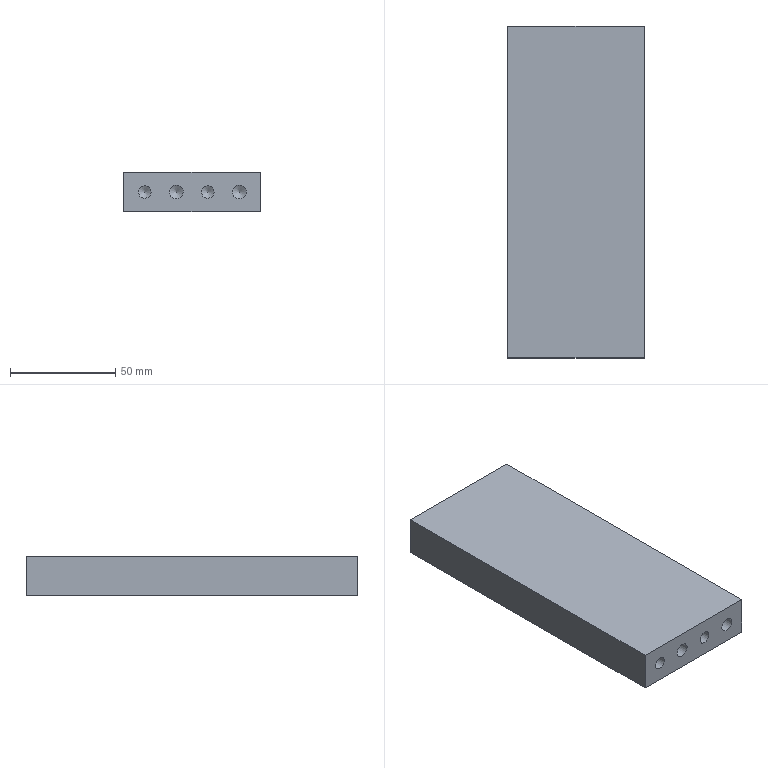Part | STEP file | SN10_006_006_SUPORTE | 1 solid | 18 faces | box 65 x 158 x 19 mm | volume 192576 mm3 | cone 6 | plane 6 | cylinder 6 | commonest cylinder face diameters 4.917 x2 6 x2 6.647 x2
STEP:
#1=CARTESIAN_POINT('',(0.,0.,0.));
#2=DIRECTION('',(0.,0.,1.));
#3=DIRECTION('',(1.,0.,0.));
#4=AXIS2_PLACEMENT_3D('',#1,#2,#3);
#5=CARTESIAN_POINT('',(286.546,-168.,375.407));
#6=VERTEX_POINT('',#5);
#7=CARTESIAN_POINT('',(283.629,-168.,377.));
#8=DIRECTION('',(0.,-1.,0.));
#9=DIRECTION('',(1.,0.,0.));
#10=AXIS2_PLACEMENT_3D('',#7,#8,#9);
#11=CIRCLE('',#10,3.324);
#12=CARTESIAN_POINT('',(283.629,-166.659,377.));
#13=DIRECTION('',(0.,-1.,0.));
#14=DIRECTION('',(0.8776,0.,-0.4794));
#15=AXIS2_PLACEMENT_3D('',#12,#13,#14);
#16=CONICAL_SURFACE('',#15,1.,1.047);
#17=CARTESIAN_POINT('',(-5.783,1.341));
#18=DIRECTION('',(1.,0.));
#19=VECTOR('',#18,1.);
#20=LINE('',#17,#19);
#21=(GEOMETRIC_REPRESENTATION_CONTEXT(2)PARAMETRIC_REPRESENTATION_CONTEXT()REPRESENTATION_CONTEXT('',''));
#22=DEFINITIONAL_REPRESENTATION('',(#20),#21);
#23=PCURVE('',#16,#22);
#24=CARTESIAN_POINT('',(283.629,-182.9,377.));
#25=DIRECTION('',(0.,1.,0.));
#26=DIRECTION('',(0.8776,0.,-0.4794));
#27=AXIS2_PLACEMENT_3D('',#24,#25,#26);
#28=CYLINDRICAL_SURFACE('',#27,3.324);
#29=CARTESIAN_POINT('',(12.066,14.9));
#30=DIRECTION('',(-1.,0.));
#31=VECTOR('',#30,1.);
#32=LINE('',#29,#31);
#33=(GEOMETRIC_REPRESENTATION_CONTEXT(2)PARAMETRIC_REPRESENTATION_CONTEXT()REPRESENTATION_CONTEXT('',''));
#34=DEFINITIONAL_REPRESENTATION('',(#32),#33);
#35=PCURVE('',#28,#34);
#36=SURFACE_CURVE('',#11,(#23,#35),.PCURVE_S1.);
#37=EDGE_CURVE('',#6,#6,#36,.T.);
#38=ORIENTED_EDGE('',*,*,#37,.F.);
#39=CARTESIAN_POINT('',(283.629,-166.081,377.));
#40=VERTEX_POINT('',#39);
#41=CARTESIAN_POINT('',(283.629,-166.081,377.));
#42=CARTESIAN_POINT('',(286.546,-168.,375.407));
#43=B_SPLINE_CURVE_WITH_KNOTS('',1,(#41,#42),.UNSPECIFIED.,.F.,.F.,(2,2),(-1.155,2.683),.PIECEWISE_BEZIER_KNOTS.);
#44=CARTESIAN_POINT('',(0.,0.));
#45=DIRECTION('',(0.,1.));
#46=VECTOR('',#45,1.);
#47=LINE('',#44,#46);
#48=(GEOMETRIC_REPRESENTATION_CONTEXT(2)PARAMETRIC_REPRESENTATION_CONTEXT()REPRESENTATION_CONTEXT('',''));
#49=DEFINITIONAL_REPRESENTATION('',(#47),#48);
#50=PCURVE('',#16,#49);
#51=CARTESIAN_POINT('',(6.283,0.));
#52=DIRECTION('',(0.,1.));
#53=VECTOR('',#52,1.);
#54=LINE('',#51,#53);
#55=(GEOMETRIC_REPRESENTATION_CONTEXT(2)PARAMETRIC_REPRESENTATION_CONTEXT()REPRESENTATION_CONTEXT('',''));
#56=DEFINITIONAL_REPRESENTATION('',(#54),#55);
#57=PCURVE('',#16,#56);
#58=SEAM_CURVE('',#43,(#50,#57),.PCURVE_S1.);
#59=EDGE_CURVE('',#40,#6,#58,.T.);
#60=ORIENTED_EDGE('',*,*,#59,.F.);
#61=ORIENTED_EDGE('',*,*,#59,.T.);
#62=EDGE_LOOP('',(#38,#60,#61));
#63=FACE_BOUND('',#62,.F.);
#64=ADVANCED_FACE('',(#63),#16,.F.);
#65=CARTESIAN_POINT('',(258.629,-183.,367.5));
#66=VERTEX_POINT('',#65);
#67=CARTESIAN_POINT('',(258.629,-25.,367.5));
#68=VERTEX_POINT('',#67);
#69=CARTESIAN_POINT('',(258.629,-183.,367.5));
#70=DIRECTION('',(0.,1.,0.));
#71=VECTOR('',#70,1.);
#72=LINE('',#69,#71);
#73=CARTESIAN_POINT('',(258.629,-183.,386.5));
#74=DIRECTION('',(-1.,0.,0.));
#75=DIRECTION('',(0.,0.,1.));
#76=AXIS2_PLACEMENT_3D('',#73,#74,#75);
#77=PLANE('',#76);
#78=CARTESIAN_POINT('',(-19.,0.));
#79=DIRECTION('',(0.,1.));
#80=VECTOR('',#79,1.);
#81=LINE('',#78,#80);
#82=(GEOMETRIC_REPRESENTATION_CONTEXT(2)PARAMETRIC_REPRESENTATION_CONTEXT()REPRESENTATION_CONTEXT('',''));
#83=DEFINITIONAL_REPRESENTATION('',(#81),#82);
#84=PCURVE('',#77,#83);
#85=CARTESIAN_POINT('',(0.,0.,367.5));
#86=DIRECTION('',(0.,0.,1.));
#87=DIRECTION('',(1.,0.,0.));
#88=AXIS2_PLACEMENT_3D('',#85,#86,#87);
#89=PLANE('',#88);
#90=CARTESIAN_POINT('',(258.629,-183.));
#91=DIRECTION('',(0.,1.));
#92=VECTOR('',#91,1.);
#93=LINE('',#90,#92);
#94=(GEOMETRIC_REPRESENTATION_CONTEXT(2)PARAMETRIC_REPRESENTATION_CONTEXT()REPRESENTATION_CONTEXT('',''));
#95=DEFINITIONAL_REPRESENTATION('',(#93),#94);
#96=PCURVE('',#89,#95);
#97=SURFACE_CURVE('',#72,(#84,#96),.PCURVE_S1.);
#98=EDGE_CURVE('',#66,#68,#97,.T.);
#99=ORIENTED_EDGE('',*,*,#98,.F.);
#100=CARTESIAN_POINT('',(258.629,-183.,386.5));
#101=VERTEX_POINT('',#100);
#102=CARTESIAN_POINT('',(258.629,-183.,386.5));
#103=DIRECTION('',(0.,0.,-1.));
#104=VECTOR('',#103,1.);
#105=LINE('',#102,#104);
#106=CARTESIAN_POINT('',(0.,0.));
#107=DIRECTION('',(-1.,0.));
#108=VECTOR('',#107,1.);
#109=LINE('',#106,#108);
#110=(GEOMETRIC_REPRESENTATION_CONTEXT(2)PARAMETRIC_REPRESENTATION_CONTEXT()REPRESENTATION_CONTEXT('',''));
#111=DEFINITIONAL_REPRESENTATION('',(#109),#110);
#112=PCURVE('',#77,#111);
#113=CARTESIAN_POINT('',(258.629,-183.,386.5));
#114=DIRECTION('',(0.,1.,0.));
#115=DIRECTION('',(0.,0.,1.));
#116=AXIS2_PLACEMENT_3D('',#113,#114,#115);
#117=PLANE('',#116);
#118=CARTESIAN_POINT('',(0.,0.));
#119=DIRECTION('',(-1.,0.));
#120=VECTOR('',#119,1.);
#121=LINE('',#118,#120);
#122=(GEOMETRIC_REPRESENTATION_CONTEXT(2)PARAMETRIC_REPRESENTATION_CONTEXT()REPRESENTATION_CONTEXT('',''));
#123=DEFINITIONAL_REPRESENTATION('',(#121),#122);
#124=PCURVE('',#117,#123);
#125=SURFACE_CURVE('',#105,(#112,#124),.PCURVE_S1.);
#126=EDGE_CURVE('',#101,#66,#125,.T.);
#127=ORIENTED_EDGE('',*,*,#126,.F.);
#128=CARTESIAN_POINT('',(258.629,-25.,386.5));
#129=VERTEX_POINT('',#128);
#130=CARTESIAN_POINT('',(258.629,-183.,386.5));
#131=DIRECTION('',(0.,1.,0.));
#132=VECTOR('',#131,1.);
#133=LINE('',#130,#132);
#134=CARTESIAN_POINT('',(0.,0.));
#135=DIRECTION('',(0.,1.));
#136=VECTOR('',#135,1.);
#137=LINE('',#134,#136);
#138=(GEOMETRIC_REPRESENTATION_CONTEXT(2)PARAMETRIC_REPRESENTATION_CONTEXT()REPRESENTATION_CONTEXT('',''));
#139=DEFINITIONAL_REPRESENTATION('',(#137),#138);
#140=PCURVE('',#77,#139);
#141=CARTESIAN_POINT('',(0.,0.,386.5));
#142=DIRECTION('',(0.,0.,1.));
#143=DIRECTION('',(1.,0.,0.));
#144=AXIS2_PLACEMENT_3D('',#141,#142,#143);
#145=PLANE('',#144);
#146=CARTESIAN_POINT('',(258.629,-183.));
#147=DIRECTION('',(0.,1.));
#148=VECTOR('',#147,1.);
#149=LINE('',#146,#148);
#150=(GEOMETRIC_REPRESENTATION_CONTEXT(2)PARAMETRIC_REPRESENTATION_CONTEXT()REPRESENTATION_CONTEXT('',''));
#151=DEFINITIONAL_REPRESENTATION('',(#149),#150);
#152=PCURVE('',#145,#151);
#153=SURFACE_CURVE('',#133,(#140,#152),.PCURVE_S1.);
#154=EDGE_CURVE('',#101,#129,#153,.T.);
#155=ORIENTED_EDGE('',*,*,#154,.T.);
#156=CARTESIAN_POINT('',(258.629,-25.,386.5));
#157=DIRECTION('',(0.,0.,-1.));
#158=VECTOR('',#157,1.);
#159=LINE('',#156,#158);
#160=CARTESIAN_POINT('',(0.,158.));
#161=DIRECTION('',(-1.,0.));
#162=VECTOR('',#161,1.);
#163=LINE('',#160,#162);
#164=(GEOMETRIC_REPRESENTATION_CONTEXT(2)PARAMETRIC_REPRESENTATION_CONTEXT()REPRESENTATION_CONTEXT('',''));
#165=DEFINITIONAL_REPRESENTATION('',(#163),#164);
#166=PCURVE('',#77,#165);
#167=CARTESIAN_POINT('',(258.629,-25.,386.5));
#168=DIRECTION('',(0.,1.,0.));
#169=DIRECTION('',(0.,0.,1.));
#170=AXIS2_PLACEMENT_3D('',#167,#168,#169);
#171=PLANE('',#170);
#172=CARTESIAN_POINT('',(0.,0.));
#173=DIRECTION('',(-1.,0.));
#174=VECTOR('',#173,1.);
#175=LINE('',#172,#174);
#176=(GEOMETRIC_REPRESENTATION_CONTEXT(2)PARAMETRIC_REPRESENTATION_CONTEXT()REPRESENTATION_CONTEXT('',''));
#177=DEFINITIONAL_REPRESENTATION('',(#175),#176);
#178=PCURVE('',#171,#177);
#179=SURFACE_CURVE('',#159,(#166,#178),.PCURVE_S1.);
#180=EDGE_CURVE('',#129,#68,#179,.T.);
#181=ORIENTED_EDGE('',*,*,#180,.T.);
#182=EDGE_LOOP('',(#99,#127,#155,#181));
#183=FACE_BOUND('',#182,.T.);
#184=ADVANCED_FACE('',(#183),#77,.T.);
#185=CARTESIAN_POINT('',(323.629,-25.,367.5));
#186=VERTEX_POINT('',#185);
#187=CARTESIAN_POINT('',(258.629,-25.,367.5));
#188=DIRECTION('',(1.,0.,0.));
#189=VECTOR('',#188,1.);
#190=LINE('',#187,#189);
#191=CARTESIAN_POINT('',(258.629,-25.));
#192=DIRECTION('',(1.,0.));
#193=VECTOR('',#192,1.);
#194=LINE('',#191,#193);
#195=(GEOMETRIC_REPRESENTATION_CONTEXT(2)PARAMETRIC_REPRESENTATION_CONTEXT()REPRESENTATION_CONTEXT('',''));
#196=DEFINITIONAL_REPRESENTATION('',(#194),#195);
#197=PCURVE('',#89,#196);
#198=CARTESIAN_POINT('',(-19.,0.));
#199=DIRECTION('',(0.,1.));
#200=VECTOR('',#199,1.);
#201=LINE('',#198,#200);
#202=(GEOMETRIC_REPRESENTATION_CONTEXT(2)PARAMETRIC_REPRESENTATION_CONTEXT()REPRESENTATION_CONTEXT('',''));
#203=DEFINITIONAL_REPRESENTATION('',(#201),#202);
#204=PCURVE('',#171,#203);
#205=SURFACE_CURVE('',#190,(#197,#204),.PCURVE_S1.);
#206=EDGE_CURVE('',#68,#186,#205,.T.);
#207=ORIENTED_EDGE('',*,*,#206,.T.);
#208=CARTESIAN_POINT('',(323.629,-183.,367.5));
#209=VERTEX_POINT('',#208);
#210=CARTESIAN_POINT('',(323.629,-25.,367.5));
#211=DIRECTION('',(0.,-1.,0.));
#212=VECTOR('',#211,1.);
#213=LINE('',#210,#212);
#214=CARTESIAN_POINT('',(323.629,-25.));
#215=DIRECTION('',(0.,-1.));
#216=VECTOR('',#215,1.);
#217=LINE('',#214,#216);
#218=(GEOMETRIC_REPRESENTATION_CONTEXT(2)PARAMETRIC_REPRESENTATION_CONTEXT()REPRESENTATION_CONTEXT('',''));
#219=DEFINITIONAL_REPRESENTATION('',(#217),#218);
#220=PCURVE('',#89,#219);
#221=CARTESIAN_POINT('',(323.629,-25.,386.5));
#222=DIRECTION('',(1.,0.,0.));
#223=DIRECTION('',(0.,0.,-1.));
#224=AXIS2_PLACEMENT_3D('',#221,#222,#223);
#225=PLANE('',#224);
#226=CARTESIAN_POINT('',(19.,0.));
#227=DIRECTION('',(0.,-1.));
#228=VECTOR('',#227,1.);
#229=LINE('',#226,#228);
#230=(GEOMETRIC_REPRESENTATION_CONTEXT(2)PARAMETRIC_REPRESENTATION_CONTEXT()REPRESENTATION_CONTEXT('',''));
#231=DEFINITIONAL_REPRESENTATION('',(#229),#230);
#232=PCURVE('',#225,#231);
#233=SURFACE_CURVE('',#213,(#220,#232),.PCURVE_S1.);
#234=EDGE_CURVE('',#186,#209,#233,.T.);
#235=ORIENTED_EDGE('',*,*,#234,.T.);
#236=CARTESIAN_POINT('',(258.629,-183.,367.5));
#237=DIRECTION('',(1.,0.,0.));
#238=VECTOR('',#237,1.);
#239=LINE('',#236,#238);
#240=CARTESIAN_POINT('',(258.629,-183.));
#241=DIRECTION('',(1.,0.));
#242=VECTOR('',#241,1.);
#243=LINE('',#240,#242);
#244=(GEOMETRIC_REPRESENTATION_CONTEXT(2)PARAMETRIC_REPRESENTATION_CONTEXT()REPRESENTATION_CONTEXT('',''));
#245=DEFINITIONAL_REPRESENTATION('',(#243),#244);
#246=PCURVE('',#89,#245);
#247=CARTESIAN_POINT('',(-19.,0.));
#248=DIRECTION('',(0.,1.));
#249=VECTOR('',#248,1.);
#250=LINE('',#247,#249);
#251=(GEOMETRIC_REPRESENTATION_CONTEXT(2)PARAMETRIC_REPRESENTATION_CONTEXT()REPRESENTATION_CONTEXT('',''));
#252=DEFINITIONAL_REPRESENTATION('',(#250),#251);
#253=PCURVE('',#117,#252);
#254=SURFACE_CURVE('',#239,(#246,#253),.PCURVE_S1.);
#255=EDGE_CURVE('',#66,#209,#254,.T.);
#256=ORIENTED_EDGE('',*,*,#255,.F.);
#257=ORIENTED_EDGE('',*,*,#98,.T.);
#258=EDGE_LOOP('',(#207,#235,#256,#257));
#259=FACE_BOUND('',#258,.T.);
#260=ADVANCED_FACE('',(#259),#89,.F.);
#261=CARTESIAN_POINT('',(301.262,-183.,375.562));
#262=VERTEX_POINT('',#261);
#263=CARTESIAN_POINT('',(298.629,-183.,377.));
#264=DIRECTION('',(0.,1.,0.));
#265=DIRECTION('',(1.,0.,0.));
#266=AXIS2_PLACEMENT_3D('',#263,#264,#265);
#267=CIRCLE('',#266,3.);
#268=CARTESIAN_POINT('',(298.629,-182.9,377.));
#269=DIRECTION('',(0.,1.,0.));
#270=DIRECTION('',(0.8776,0.,-0.4794));
#271=AXIS2_PLACEMENT_3D('',#268,#269,#270);
#272=CYLINDRICAL_SURFACE('',#271,3.);
#273=CARTESIAN_POINT('',(-0.5,-0.1));
#274=DIRECTION('',(1.,0.));
#275=VECTOR('',#274,1.);
#276=LINE('',#273,#275);
#277=(GEOMETRIC_REPRESENTATION_CONTEXT(2)PARAMETRIC_REPRESENTATION_CONTEXT()REPRESENTATION_CONTEXT('',''));
#278=DEFINITIONAL_REPRESENTATION('',(#276),#277);
#279=PCURVE('',#272,#278);
#280=CARTESIAN_POINT('',(-9.5,40.));
#281=DIRECTION('',(0.,1.));
#282=AXIS2_PLACEMENT_2D('',#280,#281);
#283=CIRCLE('',#282,3.);
#284=(GEOMETRIC_REPRESENTATION_CONTEXT(2)PARAMETRIC_REPRESENTATION_CONTEXT()REPRESENTATION_CONTEXT('',''));
#285=DEFINITIONAL_REPRESENTATION('',(#283),#284);
#286=PCURVE('',#117,#285);
#287=SURFACE_CURVE('',#267,(#279,#286),.PCURVE_S1.);
#288=EDGE_CURVE('',#262,#262,#287,.T.);
#289=ORIENTED_EDGE('',*,*,#288,.T.);
#290=CARTESIAN_POINT('',(301.262,-168.,375.562));
#291=VERTEX_POINT('',#290);
#292=CARTESIAN_POINT('',(301.262,-183.,375.562));
#293=CARTESIAN_POINT('',(301.262,-168.,375.562));
#294=B_SPLINE_CURVE_WITH_KNOTS('',1,(#292,#293),.UNSPECIFIED.,.F.,.F.,(2,2),(-0.1,14.9),.PIECEWISE_BEZIER_KNOTS.);
#295=CARTESIAN_POINT('',(6.283,0.));
#296=DIRECTION('',(0.,1.));
#297=VECTOR('',#296,1.);
#298=LINE('',#295,#297);
#299=(GEOMETRIC_REPRESENTATION_CONTEXT(2)PARAMETRIC_REPRESENTATION_CONTEXT()REPRESENTATION_CONTEXT('',''));
#300=DEFINITIONAL_REPRESENTATION('',(#298),#299);
#301=PCURVE('',#272,#300);
#302=CARTESIAN_POINT('',(0.,0.));
#303=DIRECTION('',(0.,1.));
#304=VECTOR('',#303,1.);
#305=LINE('',#302,#304);
#306=(GEOMETRIC_REPRESENTATION_CONTEXT(2)PARAMETRIC_REPRESENTATION_CONTEXT()REPRESENTATION_CONTEXT('',''));
#307=DEFINITIONAL_REPRESENTATION('',(#305),#306);
#308=PCURVE('',#272,#307);
#309=SEAM_CURVE('',#294,(#301,#308),.PCURVE_S1.);
#310=EDGE_CURVE('',#262,#291,#309,.T.);
#311=ORIENTED_EDGE('',*,*,#310,.T.);
#312=CARTESIAN_POINT('',(298.629,-168.,377.));
#313=DIRECTION('',(0.,1.,0.));
#314=DIRECTION('',(1.,0.,0.));
#315=AXIS2_PLACEMENT_3D('',#312,#313,#314);
#316=CIRCLE('',#315,3.);
#317=CARTESIAN_POINT('',(-0.5,14.9));
#318=DIRECTION('',(1.,0.));
#319=VECTOR('',#318,1.);
#320=LINE('',#317,#319);
#321=(GEOMETRIC_REPRESENTATION_CONTEXT(2)PARAMETRIC_REPRESENTATION_CONTEXT()REPRESENTATION_CONTEXT('',''));
#322=DEFINITIONAL_REPRESENTATION('',(#320),#321);
#323=PCURVE('',#272,#322);
#324=CARTESIAN_POINT('',(298.629,-166.845,377.));
#325=DIRECTION('',(0.,-1.,0.));
#326=DIRECTION('',(0.8776,0.,-0.4794));
#327=AXIS2_PLACEMENT_3D('',#324,#325,#326);
#328=CONICAL_SURFACE('',#327,1.,1.047);
#329=CARTESIAN_POINT('',(6.783,1.155));
#330=DIRECTION('',(-1.,0.));
#331=VECTOR('',#330,1.);
#332=LINE('',#329,#331);
#333=(GEOMETRIC_REPRESENTATION_CONTEXT(2)PARAMETRIC_REPRESENTATION_CONTEXT()REPRESENTATION_CONTEXT('',''));
#334=DEFINITIONAL_REPRESENTATION('',(#332),#333);
#335=PCURVE('',#328,#334);
#336=SURFACE_CURVE('',#316,(#323,#335),.PCURVE_S1.);
#337=EDGE_CURVE('',#291,#291,#336,.T.);
#338=ORIENTED_EDGE('',*,*,#337,.F.);
#339=ORIENTED_EDGE('',*,*,#310,.F.);
#340=EDGE_LOOP('',(#289,#311,#338,#339));
#341=FACE_BOUND('',#340,.F.);
#342=ADVANCED_FACE('',(#341),#272,.F.);
#343=CARTESIAN_POINT('',(265.996,-183.,378.438));
#344=VERTEX_POINT('',#343);
#345=CARTESIAN_POINT('',(268.629,-183.,377.));
#346=DIRECTION('',(0.,1.,0.));
#347=DIRECTION('',(1.,0.,0.));
#348=AXIS2_PLACEMENT_3D('',#345,#346,#347);
#349=CIRCLE('',#348,3.);
#350=CARTESIAN_POINT('',(268.629,-182.9,377.));
#351=DIRECTION('',(0.,1.,0.));
#352=DIRECTION('',(0.8776,0.,-0.4794));
#353=AXIS2_PLACEMENT_3D('',#350,#351,#352);
#354=CYLINDRICAL_SURFACE('',#353,3.);
#355=CARTESIAN_POINT('',(-0.5,-0.1));
#356=DIRECTION('',(1.,0.));
#357=VECTOR('',#356,1.);
#358=LINE('',#355,#357);
#359=(GEOMETRIC_REPRESENTATION_CONTEXT(2)PARAMETRIC_REPRESENTATION_CONTEXT()REPRESENTATION_CONTEXT('',''));
#360=DEFINITIONAL_REPRESENTATION('',(#358),#359);
#361=PCURVE('',#354,#360);
#362=CARTESIAN_POINT('',(-9.5,10.));
#363=DIRECTION('',(0.,1.));
#364=AXIS2_PLACEMENT_2D('',#362,#363);
#365=CIRCLE('',#364,3.);
#366=(GEOMETRIC_REPRESENTATION_CONTEXT(2)PARAMETRIC_REPRESENTATION_CONTEXT()REPRESENTATION_CONTEXT('',''));
#367=DEFINITIONAL_REPRESENTATION('',(#365),#366);
#368=PCURVE('',#117,#367);
#369=SURFACE_CURVE('',#349,(#361,#368),.PCURVE_S1.);
#370=EDGE_CURVE('',#344,#344,#369,.T.);
#371=ORIENTED_EDGE('',*,*,#370,.T.);
#372=CARTESIAN_POINT('',(265.996,-168.,378.438));
#373=VERTEX_POINT('',#372);
#374=CARTESIAN_POINT('',(265.996,-183.,378.438));
#375=CARTESIAN_POINT('',(265.996,-168.,378.438));
#376=B_SPLINE_CURVE_WITH_KNOTS('',1,(#374,#375),.UNSPECIFIED.,.F.,.F.,(2,2),(-0.1,14.9),.PIECEWISE_BEZIER_KNOTS.);
#377=CARTESIAN_POINT('',(9.425,0.));
#378=DIRECTION('',(0.,1.));
#379=VECTOR('',#378,1.);
#380=LINE('',#377,#379);
#381=(GEOMETRIC_REPRESENTATION_CONTEXT(2)PARAMETRIC_REPRESENTATION_CONTEXT()REPRESENTATION_CONTEXT('',''));
#382=DEFINITIONAL_REPRESENTATION('',(#380),#381);
#383=PCURVE('',#354,#382);
#384=CARTESIAN_POINT('',(3.142,0.));
#385=DIRECTION('',(0.,1.));
#386=VECTOR('',#385,1.);
#387=LINE('',#384,#386);
#388=(GEOMETRIC_REPRESENTATION_CONTEXT(2)PARAMETRIC_REPRESENTATION_CONTEXT()REPRESENTATION_CONTEXT('',''));
#389=DEFINITIONAL_REPRESENTATION('',(#387),#388);
#390=PCURVE('',#354,#389);
#391=SEAM_CURVE('',#376,(#383,#390),.PCURVE_S1.);
#392=EDGE_CURVE('',#344,#373,#391,.T.);
#393=ORIENTED_EDGE('',*,*,#392,.T.);
#394=CARTESIAN_POINT('',(268.629,-168.,377.));
#395=DIRECTION('',(0.,1.,0.));
#396=DIRECTION('',(1.,0.,0.));
#397=AXIS2_PLACEMENT_3D('',#394,#395,#396);
#398=CIRCLE('',#397,3.);
#399=CARTESIAN_POINT('',(-0.5,14.9));
#400=DIRECTION('',(1.,0.));
#401=VECTOR('',#400,1.);
#402=LINE('',#399,#401);
#403=(GEOMETRIC_REPRESENTATION_CONTEXT(2)PARAMETRIC_REPRESENTATION_CONTEXT()REPRESENTATION_CONTEXT('',''));
#404=DEFINITIONAL_REPRESENTATION('',(#402),#403);
#405=PCURVE('',#354,#404);
#406=CARTESIAN_POINT('',(268.629,-166.845,377.));
#407=DIRECTION('',(0.,-1.,0.));
#408=DIRECTION('',(0.8776,0.,-0.4794));
#409=AXIS2_PLACEMENT_3D('',#406,#407,#408);
#410=CONICAL_SURFACE('',#409,1.,1.047);
#411=CARTESIAN_POINT('',(13.066,1.155));
#412=DIRECTION('',(-1.,0.));
#413=VECTOR('',#412,1.);
#414=LINE('',#411,#413);
#415=(GEOMETRIC_REPRESENTATION_CONTEXT(2)PARAMETRIC_REPRESENTATION_CONTEXT()REPRESENTATION_CONTEXT('',''));
#416=DEFINITIONAL_REPRESENTATION('',(#414),#415);
#417=PCURVE('',#410,#416);
#418=SURFACE_CURVE('',#398,(#405,#417),.PCURVE_S1.);
#419=EDGE_CURVE('',#373,#373,#418,.T.);
#420=ORIENTED_EDGE('',*,*,#419,.F.);
#421=ORIENTED_EDGE('',*,*,#392,.F.);
#422=EDGE_LOOP('',(#371,#393,#420,#421));
#423=FACE_BOUND('',#422,.F.);
#424=ADVANCED_FACE('',(#423),#354,.F.);
#425=ORIENTED_EDGE('',*,*,#206,.F.);
#426=ORIENTED_EDGE('',*,*,#180,.F.);
#427=CARTESIAN_POINT('',(323.629,-25.,386.5));
#428=VERTEX_POINT('',#427);
#429=CARTESIAN_POINT('',(258.629,-25.,386.5));
#430=DIRECTION('',(1.,0.,0.));
#431=VECTOR('',#430,1.);
#432=LINE('',#429,#431);
#433=CARTESIAN_POINT('',(0.,0.));
#434=DIRECTION('',(0.,1.));
#435=VECTOR('',#434,1.);
#436=LINE('',#433,#435);
#437=(GEOMETRIC_REPRESENTATION_CONTEXT(2)PARAMETRIC_REPRESENTATION_CONTEXT()REPRESENTATION_CONTEXT('',''));
#438=DEFINITIONAL_REPRESENTATION('',(#436),#437);
#439=PCURVE('',#171,#438);
#440=CARTESIAN_POINT('',(258.629,-25.));
#441=DIRECTION('',(1.,0.));
#442=VECTOR('',#441,1.);
#443=LINE('',#440,#442);
#444=(GEOMETRIC_REPRESENTATION_CONTEXT(2)PARAMETRIC_REPRESENTATION_CONTEXT()REPRESENTATION_CONTEXT('',''));
#445=DEFINITIONAL_REPRESENTATION('',(#443),#444);
#446=PCURVE('',#145,#445);
#447=SURFACE_CURVE('',#432,(#439,#446),.PCURVE_S1.);
#448=EDGE_CURVE('',#129,#428,#447,.T.);
#449=ORIENTED_EDGE('',*,*,#448,.T.);
#450=CARTESIAN_POINT('',(323.629,-25.,386.5));
#451=DIRECTION('',(0.,0.,-1.));
#452=VECTOR('',#451,1.);
#453=LINE('',#450,#452);
#454=CARTESIAN_POINT('',(0.,65.));
#455=DIRECTION('',(-1.,0.));
#456=VECTOR('',#455,1.);
#457=LINE('',#454,#456);
#458=(GEOMETRIC_REPRESENTATION_CONTEXT(2)PARAMETRIC_REPRESENTATION_CONTEXT()REPRESENTATION_CONTEXT('',''));
#459=DEFINITIONAL_REPRESENTATION('',(#457),#458);
#460=PCURVE('',#171,#459);
#461=CARTESIAN_POINT('',(0.,0.));
#462=DIRECTION('',(1.,0.));
#463=VECTOR('',#462,1.);
#464=LINE('',#461,#463);
#465=(GEOMETRIC_REPRESENTATION_CONTEXT(2)PARAMETRIC_REPRESENTATION_CONTEXT()REPRESENTATION_CONTEXT('',''));
#466=DEFINITIONAL_REPRESENTATION('',(#464),#465);
#467=PCURVE('',#225,#466);
#468=SURFACE_CURVE('',#453,(#460,#467),.PCURVE_S1.);
#469=EDGE_CURVE('',#428,#186,#468,.T.);
#470=ORIENTED_EDGE('',*,*,#469,.T.);
#471=EDGE_LOOP('',(#425,#426,#449,#470));
#472=FACE_BOUND('',#471,.T.);
#473=CARTESIAN_POINT('',(313.286,-25.,379.679));
#474=VERTEX_POINT('',#473);
#475=CARTESIAN_POINT('',(311.129,-25.,378.5));
#476=DIRECTION('',(0.,1.,0.));
#477=DIRECTION('',(1.,0.,0.));
#478=AXIS2_PLACEMENT_3D('',#475,#476,#477);
#479=CIRCLE('',#478,2.458);
#480=CARTESIAN_POINT('',(-8.,52.5));
#481=DIRECTION('',(0.,1.));
#482=AXIS2_PLACEMENT_2D('',#480,#481);
#483=CIRCLE('',#482,2.458);
#484=(GEOMETRIC_REPRESENTATION_CONTEXT(2)PARAMETRIC_REPRESENTATION_CONTEXT()REPRESENTATION_CONTEXT('',''));
#485=DEFINITIONAL_REPRESENTATION('',(#483),#484);
#486=PCURVE('',#171,#485);
#487=CARTESIAN_POINT('',(311.129,-25.1,378.5));
#488=DIRECTION('',(0.,-1.,0.));
#489=DIRECTION('',(0.8776,0.,0.4794));
#490=AXIS2_PLACEMENT_3D('',#487,#488,#489);
#491=CYLINDRICAL_SURFACE('',#490,2.458);
#492=CARTESIAN_POINT('',(12.066,-0.1));
#493=DIRECTION('',(-1.,0.));
#494=VECTOR('',#493,1.);
#495=LINE('',#492,#494);
#496=(GEOMETRIC_REPRESENTATION_CONTEXT(2)PARAMETRIC_REPRESENTATION_CONTEXT()REPRESENTATION_CONTEXT('',''));
#497=DEFINITIONAL_REPRESENTATION('',(#495),#496);
#498=PCURVE('',#491,#497);
#499=SURFACE_CURVE('',#479,(#486,#498),.PCURVE_S1.);
#500=EDGE_CURVE('',#474,#474,#499,.T.);
#501=ORIENTED_EDGE('',*,*,#500,.F.);
#502=EDGE_LOOP('',(#501));
#503=FACE_BOUND('',#502,.T.);
#504=CARTESIAN_POINT('',(273.286,-25.,379.679));
#505=VERTEX_POINT('',#504);
#506=CARTESIAN_POINT('',(271.129,-25.,378.5));
#507=DIRECTION('',(0.,1.,0.));
#508=DIRECTION('',(1.,0.,0.));
#509=AXIS2_PLACEMENT_3D('',#506,#507,#508);
#510=CIRCLE('',#509,2.458);
#511=CARTESIAN_POINT('',(-8.,12.5));
#512=DIRECTION('',(0.,1.));
#513=AXIS2_PLACEMENT_2D('',#511,#512);
#514=CIRCLE('',#513,2.458);
#515=(GEOMETRIC_REPRESENTATION_CONTEXT(2)PARAMETRIC_REPRESENTATION_CONTEXT()REPRESENTATION_CONTEXT('',''));
#516=DEFINITIONAL_REPRESENTATION('',(#514),#515);
#517=PCURVE('',#171,#516);
#518=CARTESIAN_POINT('',(271.129,-25.1,378.5));
#519=DIRECTION('',(0.,-1.,0.));
#520=DIRECTION('',(0.8776,0.,0.4794));
#521=AXIS2_PLACEMENT_3D('',#518,#519,#520);
#522=CYLINDRICAL_SURFACE('',#521,2.458);
#523=CARTESIAN_POINT('',(12.066,-0.1));
#524=DIRECTION('',(-1.,0.));
#525=VECTOR('',#524,1.);
#526=LINE('',#523,#525);
#527=(GEOMETRIC_REPRESENTATION_CONTEXT(2)PARAMETRIC_REPRESENTATION_CONTEXT()REPRESENTATION_CONTEXT('',''));
#528=DEFINITIONAL_REPRESENTATION('',(#526),#527);
#529=PCURVE('',#522,#528);
#530=SURFACE_CURVE('',#510,(#517,#529),.PCURVE_S1.);
#531=EDGE_CURVE('',#505,#505,#530,.T.);
#532=ORIENTED_EDGE('',*,*,#531,.F.);
#533=EDGE_LOOP('',(#532));
#534=FACE_BOUND('',#533,.T.);
#535=ADVANCED_FACE('',(#472,#503,#534),#171,.T.);
#536=ORIENTED_EDGE('',*,*,#337,.T.);
#537=CARTESIAN_POINT('',(298.629,-166.268,377.));
#538=VERTEX_POINT('',#537);
#539=CARTESIAN_POINT('',(298.629,-166.268,377.));
#540=CARTESIAN_POINT('',(301.262,-168.,375.562));
#541=B_SPLINE_CURVE_WITH_KNOTS('',1,(#539,#540),.UNSPECIFIED.,.F.,.F.,(2,2),(-1.155,2.309),.PIECEWISE_BEZIER_KNOTS.);
#542=CARTESIAN_POINT('',(0.,0.));
#543=DIRECTION('',(0.,1.));
#544=VECTOR('',#543,1.);
#545=LINE('',#542,#544);
#546=(GEOMETRIC_REPRESENTATION_CONTEXT(2)PARAMETRIC_REPRESENTATION_CONTEXT()REPRESENTATION_CONTEXT('',''));
#547=DEFINITIONAL_REPRESENTATION('',(#545),#546);
#548=PCURVE('',#328,#547);
#549=CARTESIAN_POINT('',(6.283,0.));
#550=DIRECTION('',(0.,1.));
#551=VECTOR('',#550,1.);
#552=LINE('',#549,#551);
#553=(GEOMETRIC_REPRESENTATION_CONTEXT(2)PARAMETRIC_REPRESENTATION_CONTEXT()REPRESENTATION_CONTEXT('',''));
#554=DEFINITIONAL_REPRESENTATION('',(#552),#553);
#555=PCURVE('',#328,#554);
#556=SEAM_CURVE('',#541,(#548,#555),.PCURVE_S1.);
#557=EDGE_CURVE('',#538,#291,#556,.T.);
#558=ORIENTED_EDGE('',*,*,#557,.F.);
#559=ORIENTED_EDGE('',*,*,#557,.T.);
#560=EDGE_LOOP('',(#536,#558,#559));
#561=FACE_BOUND('',#560,.F.);
#562=ADVANCED_FACE('',(#561),#328,.F.);
#563=ORIENTED_EDGE('',*,*,#419,.T.);
#564=CARTESIAN_POINT('',(268.629,-166.268,377.));
#565=VERTEX_POINT('',#564);
#566=CARTESIAN_POINT('',(268.629,-166.268,377.));
#567=CARTESIAN_POINT('',(265.996,-168.,378.438));
#568=B_SPLINE_CURVE_WITH_KNOTS('',1,(#566,#567),.UNSPECIFIED.,.F.,.F.,(2,2),(-1.155,2.309),.PIECEWISE_BEZIER_KNOTS.);
#569=CARTESIAN_POINT('',(3.142,0.));
#570=DIRECTION('',(0.,1.));
#571=VECTOR('',#570,1.);
#572=LINE('',#569,#571);
#573=(GEOMETRIC_REPRESENTATION_CONTEXT(2)PARAMETRIC_REPRESENTATION_CONTEXT()REPRESENTATION_CONTEXT('',''));
#574=DEFINITIONAL_REPRESENTATION('',(#572),#573);
#575=PCURVE('',#410,#574);
#576=CARTESIAN_POINT('',(9.425,0.));
#577=DIRECTION('',(0.,1.));
#578=VECTOR('',#577,1.);
#579=LINE('',#576,#578);
#580=(GEOMETRIC_REPRESENTATION_CONTEXT(2)PARAMETRIC_REPRESENTATION_CONTEXT()REPRESENTATION_CONTEXT('',''));
#581=DEFINITIONAL_REPRESENTATION('',(#579),#580);
#582=PCURVE('',#410,#581);
#583=SEAM_CURVE('',#568,(#575,#582),.PCURVE_S1.);
#584=EDGE_CURVE('',#565,#373,#583,.T.);
#585=ORIENTED_EDGE('',*,*,#584,.F.);
#586=ORIENTED_EDGE('',*,*,#584,.T.);
#587=EDGE_LOOP('',(#563,#585,#586));
#588=FACE_BOUND('',#587,.F.);
#589=ADVANCED_FACE('',(#588),#410,.F.);
#590=CARTESIAN_POINT('',(313.286,-40.,379.679));
#591=VERTEX_POINT('',#590);
#592=CARTESIAN_POINT('',(311.129,-40.,378.5));
#593=DIRECTION('',(0.,1.,0.));
#594=DIRECTION('',(1.,0.,0.));
#595=AXIS2_PLACEMENT_3D('',#592,#593,#594);
#596=CIRCLE('',#595,2.458);
#597=CARTESIAN_POINT('',(311.129,-40.842,378.5));
#598=DIRECTION('',(0.,1.,0.));
#599=DIRECTION('',(0.8776,0.,0.4794));
#600=AXIS2_PLACEMENT_3D('',#597,#598,#599);
#601=CONICAL_SURFACE('',#600,1.,1.047);
#602=CARTESIAN_POINT('',(-5.783,0.8421));
#603=DIRECTION('',(1.,0.));
#604=VECTOR('',#603,1.);
#605=LINE('',#602,#604);
#606=(GEOMETRIC_REPRESENTATION_CONTEXT(2)PARAMETRIC_REPRESENTATION_CONTEXT()REPRESENTATION_CONTEXT('',''));
#607=DEFINITIONAL_REPRESENTATION('',(#605),#606);
#608=PCURVE('',#601,#607);
#609=CARTESIAN_POINT('',(12.066,14.9));
#610=DIRECTION('',(-1.,0.));
#611=VECTOR('',#610,1.);
#612=LINE('',#609,#611);
#613=(GEOMETRIC_REPRESENTATION_CONTEXT(2)PARAMETRIC_REPRESENTATION_CONTEXT()REPRESENTATION_CONTEXT('',''));
#614=DEFINITIONAL_REPRESENTATION('',(#612),#613);
#615=PCURVE('',#491,#614);
#616=SURFACE_CURVE('',#596,(#608,#615),.PCURVE_S1.);
#617=EDGE_CURVE('',#591,#591,#616,.T.);
#618=ORIENTED_EDGE('',*,*,#617,.F.);
#619=CARTESIAN_POINT('',(311.129,-41.419,378.5));
#620=VERTEX_POINT('',#619);
#621=CARTESIAN_POINT('',(311.129,-41.419,378.5));
#622=CARTESIAN_POINT('',(313.286,-40.,379.679));
#623=B_SPLINE_CURVE_WITH_KNOTS('',1,(#621,#622),.UNSPECIFIED.,.F.,.F.,(2,2),(-1.155,1.684),.PIECEWISE_BEZIER_KNOTS.);
#624=CARTESIAN_POINT('',(0.,0.));
#625=DIRECTION('',(0.,1.));
#626=VECTOR('',#625,1.);
#627=LINE('',#624,#626);
#628=(GEOMETRIC_REPRESENTATION_CONTEXT(2)PARAMETRIC_REPRESENTATION_CONTEXT()REPRESENTATION_CONTEXT('',''));
#629=DEFINITIONAL_REPRESENTATION('',(#627),#628);
#630=PCURVE('',#601,#629);
#631=CARTESIAN_POINT('',(6.283,0.));
#632=DIRECTION('',(0.,1.));
#633=VECTOR('',#632,1.);
#634=LINE('',#631,#633);
#635=(GEOMETRIC_REPRESENTATION_CONTEXT(2)PARAMETRIC_REPRESENTATION_CONTEXT()REPRESENTATION_CONTEXT('',''));
#636=DEFINITIONAL_REPRESENTATION('',(#634),#635);
#637=PCURVE('',#601,#636);
#638=SEAM_CURVE('',#623,(#630,#637),.PCURVE_S1.);
#639=EDGE_CURVE('',#620,#591,#638,.T.);
#640=ORIENTED_EDGE('',*,*,#639,.F.);
#641=ORIENTED_EDGE('',*,*,#639,.T.);
#642=EDGE_LOOP('',(#618,#640,#641));
#643=FACE_BOUND('',#642,.F.);
#644=ADVANCED_FACE('',(#643),#601,.F.);
#645=CARTESIAN_POINT('',(273.286,-40.,379.679));
#646=VERTEX_POINT('',#645);
#647=CARTESIAN_POINT('',(271.129,-40.,378.5));
#648=DIRECTION('',(0.,1.,0.));
#649=DIRECTION('',(1.,0.,0.));
#650=AXIS2_PLACEMENT_3D('',#647,#648,#649);
#651=CIRCLE('',#650,2.458);
#652=CARTESIAN_POINT('',(271.129,-40.842,378.5));
#653=DIRECTION('',(0.,1.,0.));
#654=DIRECTION('',(0.8776,0.,0.4794));
#655=AXIS2_PLACEMENT_3D('',#652,#653,#654);
#656=CONICAL_SURFACE('',#655,1.,1.047);
#657=CARTESIAN_POINT('',(-5.783,0.8421));
#658=DIRECTION('',(1.,0.));
#659=VECTOR('',#658,1.);
#660=LINE('',#657,#659);
#661=(GEOMETRIC_REPRESENTATION_CONTEXT(2)PARAMETRIC_REPRESENTATION_CONTEXT()REPRESENTATION_CONTEXT('',''));
#662=DEFINITIONAL_REPRESENTATION('',(#660),#661);
#663=PCURVE('',#656,#662);
#664=CARTESIAN_POINT('',(12.066,14.9));
#665=DIRECTION('',(-1.,0.));
#666=VECTOR('',#665,1.);
#667=LINE('',#664,#666);
#668=(GEOMETRIC_REPRESENTATION_CONTEXT(2)PARAMETRIC_REPRESENTATION_CONTEXT()REPRESENTATION_CONTEXT('',''));
#669=DEFINITIONAL_REPRESENTATION('',(#667),#668);
#670=PCURVE('',#522,#669);
#671=SURFACE_CURVE('',#651,(#663,#670),.PCURVE_S1.);
#672=EDGE_CURVE('',#646,#646,#671,.T.);
#673=ORIENTED_EDGE('',*,*,#672,.F.);
#674=CARTESIAN_POINT('',(271.129,-41.419,378.5));
#675=VERTEX_POINT('',#674);
#676=CARTESIAN_POINT('',(271.129,-41.419,378.5));
#677=CARTESIAN_POINT('',(273.286,-40.,379.679));
#678=B_SPLINE_CURVE_WITH_KNOTS('',1,(#676,#677),.UNSPECIFIED.,.F.,.F.,(2,2),(-1.155,1.684),.PIECEWISE_BEZIER_KNOTS.);
#679=CARTESIAN_POINT('',(0.,0.));
#680=DIRECTION('',(0.,1.));
#681=VECTOR('',#680,1.);
#682=LINE('',#679,#681);
#683=(GEOMETRIC_REPRESENTATION_CONTEXT(2)PARAMETRIC_REPRESENTATION_CONTEXT()REPRESENTATION_CONTEXT('',''));
#684=DEFINITIONAL_REPRESENTATION('',(#682),#683);
#685=PCURVE('',#656,#684);
#686=CARTESIAN_POINT('',(6.283,0.));
#687=DIRECTION('',(0.,1.));
#688=VECTOR('',#687,1.);
#689=LINE('',#686,#688);
#690=(GEOMETRIC_REPRESENTATION_CONTEXT(2)PARAMETRIC_REPRESENTATION_CONTEXT()REPRESENTATION_CONTEXT('',''));
#691=DEFINITIONAL_REPRESENTATION('',(#689),#690);
#692=PCURVE('',#656,#691);
#693=SEAM_CURVE('',#678,(#685,#692),.PCURVE_S1.);
#694=EDGE_CURVE('',#675,#646,#693,.T.);
#695=ORIENTED_EDGE('',*,*,#694,.F.);
#696=ORIENTED_EDGE('',*,*,#694,.T.);
#697=EDGE_LOOP('',(#673,#695,#696));
#698=FACE_BOUND('',#697,.F.);
#699=ADVANCED_FACE('',(#698),#656,.F.);
#700=ORIENTED_EDGE('',*,*,#531,.F.);
#701=CARTESIAN_POINT('',(273.286,-25.,379.679));
#702=CARTESIAN_POINT('',(273.286,-40.,379.679));
#703=B_SPLINE_CURVE_WITH_KNOTS('',1,(#701,#702),.UNSPECIFIED.,.F.,.F.,(2,2),(-0.1,14.9),.PIECEWISE_BEZIER_KNOTS.);
#704=CARTESIAN_POINT('',(6.283,0.));
#705=DIRECTION('',(0.,1.));
#706=VECTOR('',#705,1.);
#707=LINE('',#704,#706);
#708=(GEOMETRIC_REPRESENTATION_CONTEXT(2)PARAMETRIC_REPRESENTATION_CONTEXT()REPRESENTATION_CONTEXT('',''));
#709=DEFINITIONAL_REPRESENTATION('',(#707),#708);
#710=PCURVE('',#522,#709);
#711=CARTESIAN_POINT('',(0.,0.));
#712=DIRECTION('',(0.,1.));
#713=VECTOR('',#712,1.);
#714=LINE('',#711,#713);
#715=(GEOMETRIC_REPRESENTATION_CONTEXT(2)PARAMETRIC_REPRESENTATION_CONTEXT()REPRESENTATION_CONTEXT('',''));
#716=DEFINITIONAL_REPRESENTATION('',(#714),#715);
#717=PCURVE('',#522,#716);
#718=SEAM_CURVE('',#703,(#710,#717),.PCURVE_S1.);
#719=EDGE_CURVE('',#505,#646,#718,.T.);
#720=ORIENTED_EDGE('',*,*,#719,.T.);
#721=ORIENTED_EDGE('',*,*,#672,.T.);
#722=ORIENTED_EDGE('',*,*,#719,.F.);
#723=EDGE_LOOP('',(#700,#720,#721,#722));
#724=FACE_BOUND('',#723,.F.);
#725=ADVANCED_FACE('',(#724),#522,.F.);
#726=ORIENTED_EDGE('',*,*,#500,.F.);
#727=CARTESIAN_POINT('',(313.286,-25.,379.679));
#728=CARTESIAN_POINT('',(313.286,-40.,379.679));
#729=B_SPLINE_CURVE_WITH_KNOTS('',1,(#727,#728),.UNSPECIFIED.,.F.,.F.,(2,2),(-0.1,14.9),.PIECEWISE_BEZIER_KNOTS.);
#730=CARTESIAN_POINT('',(6.283,0.));
#731=DIRECTION('',(0.,1.));
#732=VECTOR('',#731,1.);
#733=LINE('',#730,#732);
#734=(GEOMETRIC_REPRESENTATION_CONTEXT(2)PARAMETRIC_REPRESENTATION_CONTEXT()REPRESENTATION_CONTEXT('',''));
#735=DEFINITIONAL_REPRESENTATION('',(#733),#734);
#736=PCURVE('',#491,#735);
#737=CARTESIAN_POINT('',(0.,0.));
#738=DIRECTION('',(0.,1.));
#739=VECTOR('',#738,1.);
#740=LINE('',#737,#739);
#741=(GEOMETRIC_REPRESENTATION_CONTEXT(2)PARAMETRIC_REPRESENTATION_CONTEXT()REPRESENTATION_CONTEXT('',''));
#742=DEFINITIONAL_REPRESENTATION('',(#740),#741);
#743=PCURVE('',#491,#742);
#744=SEAM_CURVE('',#729,(#736,#743),.PCURVE_S1.);
#745=EDGE_CURVE('',#474,#591,#744,.T.);
#746=ORIENTED_EDGE('',*,*,#745,.T.);
#747=ORIENTED_EDGE('',*,*,#617,.T.);
#748=ORIENTED_EDGE('',*,*,#745,.F.);
#749=EDGE_LOOP('',(#726,#746,#747,#748));
#750=FACE_BOUND('',#749,.F.);
#751=ADVANCED_FACE('',(#750),#491,.F.);
#752=ORIENTED_EDGE('',*,*,#234,.F.);
#753=ORIENTED_EDGE('',*,*,#469,.F.);
#754=CARTESIAN_POINT('',(323.629,-183.,386.5));
#755=VERTEX_POINT('',#754);
#756=CARTESIAN_POINT('',(323.629,-25.,386.5));
#757=DIRECTION('',(0.,-1.,0.));
#758=VECTOR('',#757,1.);
#759=LINE('',#756,#758);
#760=CARTESIAN_POINT('',(0.,0.));
#761=DIRECTION('',(0.,-1.));
#762=VECTOR('',#761,1.);
#763=LINE('',#760,#762);
#764=(GEOMETRIC_REPRESENTATION_CONTEXT(2)PARAMETRIC_REPRESENTATION_CONTEXT()REPRESENTATION_CONTEXT('',''));
#765=DEFINITIONAL_REPRESENTATION('',(#763),#764);
#766=PCURVE('',#225,#765);
#767=CARTESIAN_POINT('',(323.629,-25.));
#768=DIRECTION('',(0.,-1.));
#769=VECTOR('',#768,1.);
#770=LINE('',#767,#769);
#771=(GEOMETRIC_REPRESENTATION_CONTEXT(2)PARAMETRIC_REPRESENTATION_CONTEXT()REPRESENTATION_CONTEXT('',''));
#772=DEFINITIONAL_REPRESENTATION('',(#770),#771);
#773=PCURVE('',#145,#772);
#774=SURFACE_CURVE('',#759,(#766,#773),.PCURVE_S1.);
#775=EDGE_CURVE('',#428,#755,#774,.T.);
#776=ORIENTED_EDGE('',*,*,#775,.T.);
#777=CARTESIAN_POINT('',(323.629,-183.,386.5));
#778=DIRECTION('',(0.,0.,-1.));
#779=VECTOR('',#778,1.);
#780=LINE('',#777,#779);
#781=CARTESIAN_POINT('',(0.,-158.));
#782=DIRECTION('',(1.,0.));
#783=VECTOR('',#782,1.);
#784=LINE('',#781,#783);
#785=(GEOMETRIC_REPRESENTATION_CONTEXT(2)PARAMETRIC_REPRESENTATION_CONTEXT()REPRESENTATION_CONTEXT('',''));
#786=DEFINITIONAL_REPRESENTATION('',(#784),#785);
#787=PCURVE('',#225,#786);
#788=CARTESIAN_POINT('',(0.,65.));
#789=DIRECTION('',(-1.,0.));
#790=VECTOR('',#789,1.);
#791=LINE('',#788,#790);
#792=(GEOMETRIC_REPRESENTATION_CONTEXT(2)PARAMETRIC_REPRESENTATION_CONTEXT()REPRESENTATION_CONTEXT('',''));
#793=DEFINITIONAL_REPRESENTATION('',(#791),#792);
#794=PCURVE('',#117,#793);
#795=SURFACE_CURVE('',#780,(#787,#794),.PCURVE_S1.);
#796=EDGE_CURVE('',#755,#209,#795,.T.);
#797=ORIENTED_EDGE('',*,*,#796,.T.);
#798=EDGE_LOOP('',(#752,#753,#776,#797));
#799=FACE_BOUND('',#798,.T.);
#800=ADVANCED_FACE('',(#799),#225,.T.);
#801=ORIENTED_EDGE('',*,*,#154,.F.);
#802=CARTESIAN_POINT('',(258.629,-183.,386.5));
#803=DIRECTION('',(1.,0.,0.));
#804=VECTOR('',#803,1.);
#805=LINE('',#802,#804);
#806=CARTESIAN_POINT('',(258.629,-183.));
#807=DIRECTION('',(1.,0.));
#808=VECTOR('',#807,1.);
#809=LINE('',#806,#808);
#810=(GEOMETRIC_REPRESENTATION_CONTEXT(2)PARAMETRIC_REPRESENTATION_CONTEXT()REPRESENTATION_CONTEXT('',''));
#811=DEFINITIONAL_REPRESENTATION('',(#809),#810);
#812=PCURVE('',#145,#811);
#813=CARTESIAN_POINT('',(0.,0.));
#814=DIRECTION('',(0.,1.));
#815=VECTOR('',#814,1.);
#816=LINE('',#813,#815);
#817=(GEOMETRIC_REPRESENTATION_CONTEXT(2)PARAMETRIC_REPRESENTATION_CONTEXT()REPRESENTATION_CONTEXT('',''));
#818=DEFINITIONAL_REPRESENTATION('',(#816),#817);
#819=PCURVE('',#117,#818);
#820=SURFACE_CURVE('',#805,(#812,#819),.PCURVE_S1.);
#821=EDGE_CURVE('',#101,#755,#820,.T.);
#822=ORIENTED_EDGE('',*,*,#821,.T.);
#823=ORIENTED_EDGE('',*,*,#775,.F.);
#824=ORIENTED_EDGE('',*,*,#448,.F.);
#825=EDGE_LOOP('',(#801,#822,#823,#824));
#826=FACE_BOUND('',#825,.T.);
#827=ADVANCED_FACE('',(#826),#145,.T.);
#828=CARTESIAN_POINT('',(286.546,-183.,375.407));
#829=VERTEX_POINT('',#828);
#830=CARTESIAN_POINT('',(283.629,-183.,377.));
#831=DIRECTION('',(0.,1.,0.));
#832=DIRECTION('',(1.,0.,0.));
#833=AXIS2_PLACEMENT_3D('',#830,#831,#832);
#834=CIRCLE('',#833,3.324);
#835=CARTESIAN_POINT('',(-0.5,-0.1));
#836=DIRECTION('',(1.,0.));
#837=VECTOR('',#836,1.);
#838=LINE('',#835,#837);
#839=(GEOMETRIC_REPRESENTATION_CONTEXT(2)PARAMETRIC_REPRESENTATION_CONTEXT()REPRESENTATION_CONTEXT('',''));
#840=DEFINITIONAL_REPRESENTATION('',(#838),#839);
#841=PCURVE('',#28,#840);
#842=CARTESIAN_POINT('',(-9.5,25.));
#843=DIRECTION('',(0.,1.));
#844=AXIS2_PLACEMENT_2D('',#842,#843);
#845=CIRCLE('',#844,3.324);
#846=(GEOMETRIC_REPRESENTATION_CONTEXT(2)PARAMETRIC_REPRESENTATION_CONTEXT()REPRESENTATION_CONTEXT('',''));
#847=DEFINITIONAL_REPRESENTATION('',(#845),#846);
#848=PCURVE('',#117,#847);
#849=SURFACE_CURVE('',#834,(#841,#848),.PCURVE_S1.);
#850=EDGE_CURVE('',#829,#829,#849,.T.);
#851=ORIENTED_EDGE('',*,*,#850,.T.);
#852=CARTESIAN_POINT('',(286.546,-183.,375.407));
#853=CARTESIAN_POINT('',(286.546,-168.,375.407));
#854=B_SPLINE_CURVE_WITH_KNOTS('',1,(#852,#853),.UNSPECIFIED.,.F.,.F.,(2,2),(-0.1,14.9),.PIECEWISE_BEZIER_KNOTS.);
#855=CARTESIAN_POINT('',(6.283,0.));
#856=DIRECTION('',(0.,1.));
#857=VECTOR('',#856,1.);
#858=LINE('',#855,#857);
#859=(GEOMETRIC_REPRESENTATION_CONTEXT(2)PARAMETRIC_REPRESENTATION_CONTEXT()REPRESENTATION_CONTEXT('',''));
#860=DEFINITIONAL_REPRESENTATION('',(#858),#859);
#861=PCURVE('',#28,#860);
#862=CARTESIAN_POINT('',(0.,0.));
#863=DIRECTION('',(0.,1.));
#864=VECTOR('',#863,1.);
#865=LINE('',#862,#864);
#866=(GEOMETRIC_REPRESENTATION_CONTEXT(2)PARAMETRIC_REPRESENTATION_CONTEXT()REPRESENTATION_CONTEXT('',''));
#867=DEFINITIONAL_REPRESENTATION('',(#865),#866);
#868=PCURVE('',#28,#867);
#869=SEAM_CURVE('',#854,(#861,#868),.PCURVE_S1.);
#870=EDGE_CURVE('',#829,#6,#869,.T.);
#871=ORIENTED_EDGE('',*,*,#870,.T.);
#872=ORIENTED_EDGE('',*,*,#37,.T.);
#873=ORIENTED_EDGE('',*,*,#870,.F.);
#874=EDGE_LOOP('',(#851,#871,#872,#873));
#875=FACE_BOUND('',#874,.F.);
#876=ADVANCED_FACE('',(#875),#28,.F.);
#877=ORIENTED_EDGE('',*,*,#255,.T.);
#878=ORIENTED_EDGE('',*,*,#796,.F.);
#879=ORIENTED_EDGE('',*,*,#821,.F.);
#880=ORIENTED_EDGE('',*,*,#126,.T.);
#881=EDGE_LOOP('',(#877,#878,#879,#880));
#882=FACE_BOUND('',#881,.T.);
#883=CARTESIAN_POINT('',(310.712,-183.,378.593));
#884=VERTEX_POINT('',#883);
#885=CARTESIAN_POINT('',(316.546,-183.,375.407));
#886=VERTEX_POINT('',#885);
#887=CARTESIAN_POINT('',(313.629,-183.,377.));
#888=DIRECTION('',(0.,1.,0.));
#889=DIRECTION('',(1.,0.,0.));
#890=AXIS2_PLACEMENT_3D('',#887,#888,#889);
#891=CIRCLE('',#890,3.324);
#892=CARTESIAN_POINT('',(-9.5,55.));
#893=DIRECTION('',(0.,1.));
#894=AXIS2_PLACEMENT_2D('',#892,#893);
#895=CIRCLE('',#894,3.324);
#896=(GEOMETRIC_REPRESENTATION_CONTEXT(2)PARAMETRIC_REPRESENTATION_CONTEXT()REPRESENTATION_CONTEXT('',''));
#897=DEFINITIONAL_REPRESENTATION('',(#895),#896);
#898=PCURVE('',#117,#897);
#899=CARTESIAN_POINT('',(313.629,-182.9,377.));
#900=DIRECTION('',(0.,1.,0.));
#901=DIRECTION('',(0.8776,0.,-0.4794));
#902=AXIS2_PLACEMENT_3D('',#899,#900,#901);
#903=CYLINDRICAL_SURFACE('',#902,3.324);
#904=CARTESIAN_POINT('',(-0.5,-0.1));
#905=DIRECTION('',(1.,0.));
#906=VECTOR('',#905,1.);
#907=LINE('',#904,#906);
#908=(GEOMETRIC_REPRESENTATION_CONTEXT(2)PARAMETRIC_REPRESENTATION_CONTEXT()REPRESENTATION_CONTEXT('',''));
#909=DEFINITIONAL_REPRESENTATION('',(#907),#908);
#910=PCURVE('',#903,#909);
#911=SURFACE_CURVE('',#891,(#898,#910),.PCURVE_S1.);
#912=EDGE_CURVE('',#884,#886,#911,.T.);
#913=ORIENTED_EDGE('',*,*,#912,.T.);
#914=CARTESIAN_POINT('',(313.629,-183.,377.));
#915=DIRECTION('',(0.,1.,0.));
#916=DIRECTION('',(1.,0.,0.));
#917=AXIS2_PLACEMENT_3D('',#914,#915,#916);
#918=CIRCLE('',#917,3.324);
#919=CARTESIAN_POINT('',(-9.5,55.));
#920=DIRECTION('',(0.,1.));
#921=AXIS2_PLACEMENT_2D('',#919,#920);
#922=CIRCLE('',#921,3.324);
#923=(GEOMETRIC_REPRESENTATION_CONTEXT(2)PARAMETRIC_REPRESENTATION_CONTEXT()REPRESENTATION_CONTEXT('',''));
#924=DEFINITIONAL_REPRESENTATION('',(#922),#923);
#925=PCURVE('',#117,#924);
#926=CARTESIAN_POINT('',(-0.5,-0.1));
#927=DIRECTION('',(1.,0.));
#928=VECTOR('',#927,1.);
#929=LINE('',#926,#928);
#930=(GEOMETRIC_REPRESENTATION_CONTEXT(2)PARAMETRIC_REPRESENTATION_CONTEXT()REPRESENTATION_CONTEXT('',''));
#931=DEFINITIONAL_REPRESENTATION('',(#929),#930);
#932=PCURVE('',#903,#931);
#933=SURFACE_CURVE('',#918,(#925,#932),.PCURVE_S1.);
#934=EDGE_CURVE('',#886,#884,#933,.T.);
#935=ORIENTED_EDGE('',*,*,#934,.T.);
#936=EDGE_LOOP('',(#913,#935));
#937=FACE_BOUND('',#936,.T.);
#938=ORIENTED_EDGE('',*,*,#850,.T.);
#939=EDGE_LOOP('',(#938));
#940=FACE_BOUND('',#939,.T.);
#941=ORIENTED_EDGE('',*,*,#288,.T.);
#942=EDGE_LOOP('',(#941));
#943=FACE_BOUND('',#942,.T.);
#944=ORIENTED_EDGE('',*,*,#370,.T.);
#945=EDGE_LOOP('',(#944));
#946=FACE_BOUND('',#945,.T.);
#947=ADVANCED_FACE('',(#882,#937,#940,#943,#946),#117,.F.);
#948=CARTESIAN_POINT('',(316.546,-168.,375.407));
#949=VERTEX_POINT('',#948);
#950=CARTESIAN_POINT('',(313.629,-168.,377.));
#951=DIRECTION('',(0.,-1.,0.));
#952=DIRECTION('',(1.,0.,0.));
#953=AXIS2_PLACEMENT_3D('',#950,#951,#952);
#954=CIRCLE('',#953,3.324);
#955=CARTESIAN_POINT('',(313.629,-166.659,377.));
#956=DIRECTION('',(0.,-1.,0.));
#957=DIRECTION('',(0.8776,0.,-0.4794));
#958=AXIS2_PLACEMENT_3D('',#955,#956,#957);
#959=CONICAL_SURFACE('',#958,1.,1.047);
#960=CARTESIAN_POINT('',(-5.783,1.341));
#961=DIRECTION('',(1.,0.));
#962=VECTOR('',#961,1.);
#963=LINE('',#960,#962);
#964=(GEOMETRIC_REPRESENTATION_CONTEXT(2)PARAMETRIC_REPRESENTATION_CONTEXT()REPRESENTATION_CONTEXT('',''));
#965=DEFINITIONAL_REPRESENTATION('',(#963),#964);
#966=PCURVE('',#959,#965);
#967=CARTESIAN_POINT('',(12.066,14.9));
#968=DIRECTION('',(-1.,0.));
#969=VECTOR('',#968,1.);
#970=LINE('',#967,#969);
#971=(GEOMETRIC_REPRESENTATION_CONTEXT(2)PARAMETRIC_REPRESENTATION_CONTEXT()REPRESENTATION_CONTEXT('',''));
#972=DEFINITIONAL_REPRESENTATION('',(#970),#971);
#973=PCURVE('',#903,#972);
#974=SURFACE_CURVE('',#954,(#966,#973),.PCURVE_S1.);
#975=EDGE_CURVE('',#949,#949,#974,.T.);
#976=ORIENTED_EDGE('',*,*,#975,.F.);
#977=CARTESIAN_POINT('',(313.629,-166.081,377.));
#978=VERTEX_POINT('',#977);
#979=CARTESIAN_POINT('',(313.629,-166.081,377.));
#980=CARTESIAN_POINT('',(316.546,-168.,375.407));
#981=B_SPLINE_CURVE_WITH_KNOTS('',1,(#979,#980),.UNSPECIFIED.,.F.,.F.,(2,2),(-1.155,2.683),.PIECEWISE_BEZIER_KNOTS.);
#982=CARTESIAN_POINT('',(0.,0.));
#983=DIRECTION('',(0.,1.));
#984=VECTOR('',#983,1.);
#985=LINE('',#982,#984);
#986=(GEOMETRIC_REPRESENTATION_CONTEXT(2)PARAMETRIC_REPRESENTATION_CONTEXT()REPRESENTATION_CONTEXT('',''));
#987=DEFINITIONAL_REPRESENTATION('',(#985),#986);
#988=PCURVE('',#959,#987);
#989=CARTESIAN_POINT('',(6.283,0.));
#990=DIRECTION('',(0.,1.));
#991=VECTOR('',#990,1.);
#992=LINE('',#989,#991);
#993=(GEOMETRIC_REPRESENTATION_CONTEXT(2)PARAMETRIC_REPRESENTATION_CONTEXT()REPRESENTATION_CONTEXT('',''));
#994=DEFINITIONAL_REPRESENTATION('',(#992),#993);
#995=PCURVE('',#959,#994);
#996=SEAM_CURVE('',#981,(#988,#995),.PCURVE_S1.);
#997=EDGE_CURVE('',#978,#949,#996,.T.);
#998=ORIENTED_EDGE('',*,*,#997,.F.);
#999=ORIENTED_EDGE('',*,*,#997,.T.);
#1000=EDGE_LOOP('',(#976,#998,#999));
#1001=FACE_BOUND('',#1000,.F.);
#1002=ADVANCED_FACE('',(#1001),#959,.F.);
#1003=ORIENTED_EDGE('',*,*,#912,.T.);
#1004=CARTESIAN_POINT('',(316.546,-183.,375.407));
#1005=CARTESIAN_POINT('',(316.546,-168.,375.407));
#1006=B_SPLINE_CURVE_WITH_KNOTS('',1,(#1004,#1005),.UNSPECIFIED.,.F.,.F.,(2,2),(-0.1,14.9),.PIECEWISE_BEZIER_KNOTS.);
#1007=CARTESIAN_POINT('',(6.283,0.));
#1008=DIRECTION('',(0.,1.));
#1009=VECTOR('',#1008,1.);
#1010=LINE('',#1007,#1009);
#1011=(GEOMETRIC_REPRESENTATION_CONTEXT(2)PARAMETRIC_REPRESENTATION_CONTEXT()REPRESENTATION_CONTEXT('',''));
#1012=DEFINITIONAL_REPRESENTATION('',(#1010),#1011);
#1013=PCURVE('',#903,#1012);
#1014=CARTESIAN_POINT('',(0.,0.));
#1015=DIRECTION('',(0.,1.));
#1016=VECTOR('',#1015,1.);
#1017=LINE('',#1014,#1016);
#1018=(GEOMETRIC_REPRESENTATION_CONTEXT(2)PARAMETRIC_REPRESENTATION_CONTEXT()REPRESENTATION_CONTEXT('',''));
#1019=DEFINITIONAL_REPRESENTATION('',(#1017),#1018);
#1020=PCURVE('',#903,#1019);
#1021=SEAM_CURVE('',#1006,(#1013,#1020),.PCURVE_S1.);
#1022=EDGE_CURVE('',#886,#949,#1021,.T.);
#1023=ORIENTED_EDGE('',*,*,#1022,.T.);
#1024=ORIENTED_EDGE('',*,*,#975,.T.);
#1025=ORIENTED_EDGE('',*,*,#1022,.F.);
#1026=ORIENTED_EDGE('',*,*,#934,.T.);
#1027=EDGE_LOOP('',(#1003,#1023,#1024,#1025,#1026));
#1028=FACE_BOUND('',#1027,.F.);
#1029=ADVANCED_FACE('',(#1028),#903,.F.);
#1030=CLOSED_SHELL('',(#64,#184,#260,#342,#424,#535,#562,#589,#644,#699,#725,#751,#800,#827,#876,#947,#1002,#1029));
#1031=MANIFOLD_SOLID_BREP('',#1030);
#1032=(LENGTH_UNIT()NAMED_UNIT(*)SI_UNIT(.MILLI.,.METRE.));
#1033=UNCERTAINTY_MEASURE_WITH_UNIT(LENGTH_MEASURE(0.000005),#1032,'','');
#1034=(NAMED_UNIT(*)PLANE_ANGLE_UNIT()SI_UNIT($,.RADIAN.));
#1035=(NAMED_UNIT(*)SI_UNIT($,.STERADIAN.)SOLID_ANGLE_UNIT());
#1036=(GEOMETRIC_REPRESENTATION_CONTEXT(3)GLOBAL_UNCERTAINTY_ASSIGNED_CONTEXT((#1033))GLOBAL_UNIT_ASSIGNED_CONTEXT((#1032,#1034,#1035))REPRESENTATION_CONTEXT('',''));
#1037=ADVANCED_BREP_SHAPE_REPRESENTATION('',(#4,#1031),#1036);